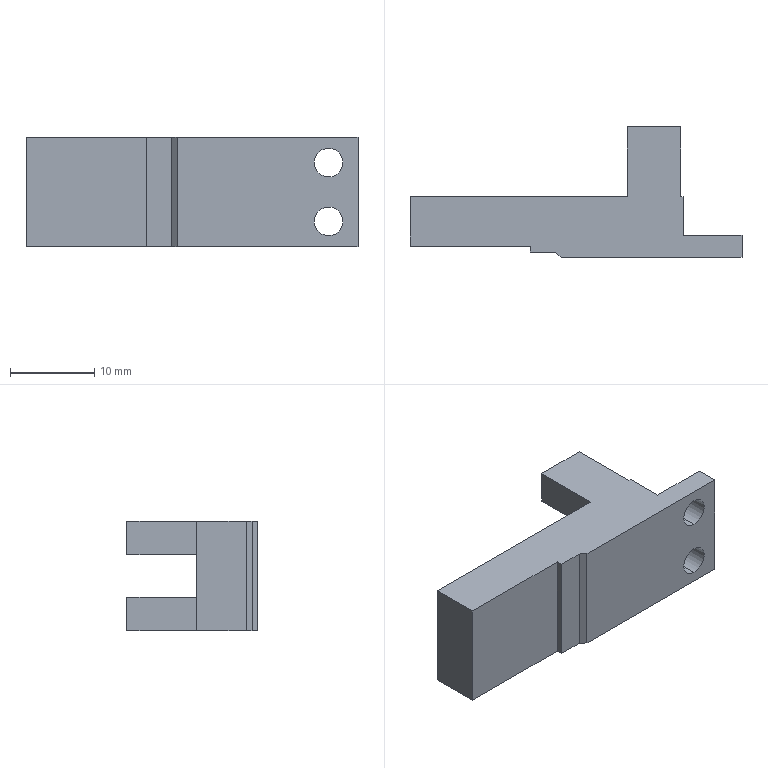Part | SolidWorks | features BaseBody 1 | 1 solid | 24 faces | box 39.5 x 15.5 x 13 mm | volume 3385 mm3 | plane 20 | cylinder 4 | commonest cylinder face diameters 3.4 x4
STEP:
#1=CARTESIAN_POINT('',(93.5,24.1,-79.8));
#2=VERTEX_POINT('',#1);
#3=CARTESIAN_POINT('',(93.5,24.1,-83.2));
#4=VERTEX_POINT('',#3);
#5=CARTESIAN_POINT('',(93.5,24.1,-81.5));
#6=DIRECTION('',(0.,-1.,0.));
#7=DIRECTION('',(0.,0.,-1.));
#8=AXIS2_PLACEMENT_3D('',#5,#6,#7);
#9=CIRCLE('',#8,1.7);
#10=EDGE_CURVE('',#2,#4,#9,.T.);
#11=ORIENTED_EDGE('',*,*,#10,.F.);
#12=CARTESIAN_POINT('',(93.5,21.5,-79.8));
#13=VERTEX_POINT('',#12);
#14=CARTESIAN_POINT('',(93.5,14.1,-79.8));
#15=DIRECTION('',(0.,-1.,0.));
#16=VECTOR('',#15,1000.);
#17=LINE('',#14,#16);
#18=EDGE_CURVE('',#2,#13,#17,.T.);
#19=ORIENTED_EDGE('',*,*,#18,.T.);
#20=CARTESIAN_POINT('',(93.5,21.5,-83.2));
#21=VERTEX_POINT('',#20);
#22=CARTESIAN_POINT('',(93.5,21.5,-81.5));
#23=DIRECTION('',(0.,1.,0.));
#24=DIRECTION('',(0.,0.,-1.));
#25=AXIS2_PLACEMENT_3D('',#22,#23,#24);
#26=CIRCLE('',#25,1.7);
#27=EDGE_CURVE('',#21,#13,#26,.T.);
#28=ORIENTED_EDGE('',*,*,#27,.F.);
#29=CARTESIAN_POINT('',(93.5,14.1,-83.2));
#30=DIRECTION('',(0.,-1.,0.));
#31=VECTOR('',#30,1000.);
#32=LINE('',#29,#31);
#33=EDGE_CURVE('',#4,#21,#32,.T.);
#34=ORIENTED_EDGE('',*,*,#33,.F.);
#35=EDGE_LOOP('',(#11,#19,#28,#34));
#36=FACE_OUTER_BOUND('',#35,.T.);
#37=CARTESIAN_POINT('',(93.5,14.1,-81.5));
#38=DIRECTION('',(0.,-1.,0.));
#39=DIRECTION('',(0.,0.,-1.));
#40=AXIS2_PLACEMENT_3D('',#37,#38,#39);
#41=CYLINDRICAL_SURFACE('',#40,1.7);
#42=ADVANCED_FACE('',(#36),#41,.F.);
#43=CARTESIAN_POINT('',(93.5,24.1,-72.8));
#44=VERTEX_POINT('',#43);
#45=CARTESIAN_POINT('',(93.5,24.1,-76.2));
#46=VERTEX_POINT('',#45);
#47=CARTESIAN_POINT('',(93.5,24.1,-74.5));
#48=DIRECTION('',(0.,-1.,0.));
#49=DIRECTION('',(0.,0.,-1.));
#50=AXIS2_PLACEMENT_3D('',#47,#48,#49);
#51=CIRCLE('',#50,1.7);
#52=EDGE_CURVE('',#44,#46,#51,.T.);
#53=ORIENTED_EDGE('',*,*,#52,.F.);
#54=CARTESIAN_POINT('',(93.5,21.5,-72.8));
#55=VERTEX_POINT('',#54);
#56=CARTESIAN_POINT('',(93.5,14.1,-72.8));
#57=DIRECTION('',(0.,-1.,0.));
#58=VECTOR('',#57,1000.);
#59=LINE('',#56,#58);
#60=EDGE_CURVE('',#44,#55,#59,.T.);
#61=ORIENTED_EDGE('',*,*,#60,.T.);
#62=CARTESIAN_POINT('',(93.5,21.5,-76.2));
#63=VERTEX_POINT('',#62);
#64=CARTESIAN_POINT('',(93.5,21.5,-74.5));
#65=DIRECTION('',(0.,1.,0.));
#66=DIRECTION('',(0.,0.,-1.));
#67=AXIS2_PLACEMENT_3D('',#64,#65,#66);
#68=CIRCLE('',#67,1.7);
#69=EDGE_CURVE('',#63,#55,#68,.T.);
#70=ORIENTED_EDGE('',*,*,#69,.F.);
#71=CARTESIAN_POINT('',(93.5,14.1,-76.2));
#72=DIRECTION('',(0.,-1.,0.));
#73=VECTOR('',#72,1000.);
#74=LINE('',#71,#73);
#75=EDGE_CURVE('',#46,#63,#74,.T.);
#76=ORIENTED_EDGE('',*,*,#75,.F.);
#77=EDGE_LOOP('',(#53,#61,#70,#76));
#78=FACE_OUTER_BOUND('',#77,.T.);
#79=CARTESIAN_POINT('',(93.5,14.1,-74.5));
#80=DIRECTION('',(0.,-1.,0.));
#81=DIRECTION('',(0.,0.,-1.));
#82=AXIS2_PLACEMENT_3D('',#79,#80,#81);
#83=CYLINDRICAL_SURFACE('',#82,1.7);
#84=ADVANCED_FACE('',(#78),#83,.F.);
#85=CARTESIAN_POINT('',(57.5,28.7,-84.5));
#86=VERTEX_POINT('',#85);
#87=CARTESIAN_POINT('',(57.5,28.7,-71.5));
#88=VERTEX_POINT('',#87);
#89=CARTESIAN_POINT('',(57.5,28.7,-84.5));
#90=DIRECTION('',(0.,0.,1.));
#91=VECTOR('',#90,1000.);
#92=LINE('',#89,#91);
#93=EDGE_CURVE('',#86,#88,#92,.T.);
#94=ORIENTED_EDGE('',*,*,#93,.T.);
#95=CARTESIAN_POINT('',(83.35,28.7,-71.5));
#96=VERTEX_POINT('',#95);
#97=CARTESIAN_POINT('',(83.35,28.7,-71.5));
#98=DIRECTION('',(1.,0.,0.));
#99=VECTOR('',#98,1000.);
#100=LINE('',#97,#99);
#101=EDGE_CURVE('',#88,#96,#100,.T.);
#102=ORIENTED_EDGE('',*,*,#101,.T.);
#103=CARTESIAN_POINT('',(83.35,28.7,-75.5));
#104=VERTEX_POINT('',#103);
#105=CARTESIAN_POINT('',(83.35,28.7,-84.5));
#106=DIRECTION('',(0.,0.,-1.));
#107=VECTOR('',#106,1000.);
#108=LINE('',#105,#107);
#109=EDGE_CURVE('',#96,#104,#108,.T.);
#110=ORIENTED_EDGE('',*,*,#109,.T.);
#111=CARTESIAN_POINT('',(89.7,28.7,-75.5));
#112=VERTEX_POINT('',#111);
#113=CARTESIAN_POINT('',(83.35,28.7,-75.5));
#114=DIRECTION('',(1.,0.,0.));
#115=VECTOR('',#114,1000.);
#116=LINE('',#113,#115);
#117=EDGE_CURVE('',#104,#112,#116,.T.);
#118=ORIENTED_EDGE('',*,*,#117,.T.);
#119=CARTESIAN_POINT('',(89.7,28.7,-71.5));
#120=VERTEX_POINT('',#119);
#121=CARTESIAN_POINT('',(89.7,28.7,-84.5));
#122=DIRECTION('',(0.,0.,1.));
#123=VECTOR('',#122,1000.);
#124=LINE('',#121,#123);
#125=EDGE_CURVE('',#112,#120,#124,.T.);
#126=ORIENTED_EDGE('',*,*,#125,.T.);
#127=CARTESIAN_POINT('',(90.,28.7,-71.5));
#128=VERTEX_POINT('',#127);
#129=CARTESIAN_POINT('',(83.35,28.7,-71.5));
#130=DIRECTION('',(1.,0.,0.));
#131=VECTOR('',#130,1000.);
#132=LINE('',#129,#131);
#133=EDGE_CURVE('',#120,#128,#132,.T.);
#134=ORIENTED_EDGE('',*,*,#133,.T.);
#135=CARTESIAN_POINT('',(90.,28.7,-84.5));
#136=VERTEX_POINT('',#135);
#137=CARTESIAN_POINT('',(90.,28.7,-84.5));
#138=DIRECTION('',(0.,0.,-1.));
#139=VECTOR('',#138,1000.);
#140=LINE('',#137,#139);
#141=EDGE_CURVE('',#128,#136,#140,.T.);
#142=ORIENTED_EDGE('',*,*,#141,.T.);
#143=CARTESIAN_POINT('',(89.7,28.7,-84.5));
#144=VERTEX_POINT('',#143);
#145=CARTESIAN_POINT('',(83.35,28.7,-84.5));
#146=DIRECTION('',(-1.,0.,0.));
#147=VECTOR('',#146,1000.);
#148=LINE('',#145,#147);
#149=EDGE_CURVE('',#136,#144,#148,.T.);
#150=ORIENTED_EDGE('',*,*,#149,.T.);
#151=CARTESIAN_POINT('',(89.7,28.7,-80.5));
#152=VERTEX_POINT('',#151);
#153=CARTESIAN_POINT('',(89.7,28.7,-84.5));
#154=DIRECTION('',(0.,0.,1.));
#155=VECTOR('',#154,1000.);
#156=LINE('',#153,#155);
#157=EDGE_CURVE('',#144,#152,#156,.T.);
#158=ORIENTED_EDGE('',*,*,#157,.T.);
#159=CARTESIAN_POINT('',(83.35,28.7,-80.5));
#160=VERTEX_POINT('',#159);
#161=CARTESIAN_POINT('',(83.35,28.7,-80.5));
#162=DIRECTION('',(-1.,0.,0.));
#163=VECTOR('',#162,1000.);
#164=LINE('',#161,#163);
#165=EDGE_CURVE('',#152,#160,#164,.T.);
#166=ORIENTED_EDGE('',*,*,#165,.T.);
#167=CARTESIAN_POINT('',(83.35,28.7,-84.5));
#168=VERTEX_POINT('',#167);
#169=CARTESIAN_POINT('',(83.35,28.7,-84.5));
#170=DIRECTION('',(0.,0.,-1.));
#171=VECTOR('',#170,1000.);
#172=LINE('',#169,#171);
#173=EDGE_CURVE('',#160,#168,#172,.T.);
#174=ORIENTED_EDGE('',*,*,#173,.T.);
#175=CARTESIAN_POINT('',(83.35,28.7,-84.5));
#176=DIRECTION('',(-1.,0.,0.));
#177=VECTOR('',#176,1000.);
#178=LINE('',#175,#177);
#179=EDGE_CURVE('',#168,#86,#178,.T.);
#180=ORIENTED_EDGE('',*,*,#179,.T.);
#181=EDGE_LOOP('',(#94,#102,#110,#118,#126,#134,#142,#150,#158,#166,#174,#180));
#182=FACE_OUTER_BOUND('',#181,.T.);
#183=CARTESIAN_POINT('',(83.35,28.7,-84.5));
#184=DIRECTION('',(0.,1.,0.));
#185=DIRECTION('',(0.,0.,1.));
#186=AXIS2_PLACEMENT_3D('',#183,#184,#185);
#187=PLANE('',#186);
#188=ADVANCED_FACE('',(#182),#187,.T.);
#189=CARTESIAN_POINT('',(83.35,37.,-71.5));
#190=VERTEX_POINT('',#189);
#191=CARTESIAN_POINT('',(83.35,0.,-71.5));
#192=DIRECTION('',(0.,-1.,0.));
#193=VECTOR('',#192,1000.);
#194=LINE('',#191,#193);
#195=EDGE_CURVE('',#190,#96,#194,.T.);
#196=ORIENTED_EDGE('',*,*,#195,.T.);
#197=ORIENTED_EDGE('',*,*,#101,.F.);
#198=CARTESIAN_POINT('',(57.5,22.8,-71.5));
#199=VERTEX_POINT('',#198);
#200=CARTESIAN_POINT('',(57.5,0.,-71.5));
#201=DIRECTION('',(0.,-1.,0.));
#202=VECTOR('',#201,1000.);
#203=LINE('',#200,#202);
#204=EDGE_CURVE('',#88,#199,#203,.T.);
#205=ORIENTED_EDGE('',*,*,#204,.T.);
#206=CARTESIAN_POINT('',(71.8,22.8,-71.5));
#207=VERTEX_POINT('',#206);
#208=CARTESIAN_POINT('',(0.,22.8,-71.5));
#209=DIRECTION('',(1.,0.,0.));
#210=VECTOR('',#209,1000.);
#211=LINE('',#208,#210);
#212=EDGE_CURVE('',#199,#207,#211,.T.);
#213=ORIENTED_EDGE('',*,*,#212,.T.);
#214=CARTESIAN_POINT('',(71.8,22.1,-71.5));
#215=VERTEX_POINT('',#214);
#216=CARTESIAN_POINT('',(71.8,22.8,-71.5));
#217=DIRECTION('',(0.,1.,0.));
#218=VECTOR('',#217,1000.);
#219=LINE('',#216,#218);
#220=EDGE_CURVE('',#215,#207,#219,.T.);
#221=ORIENTED_EDGE('',*,*,#220,.F.);
#222=CARTESIAN_POINT('',(74.8,22.1,-71.5));
#223=VERTEX_POINT('',#222);
#224=CARTESIAN_POINT('',(0.,22.1,-71.5));
#225=DIRECTION('',(1.,0.,0.));
#226=VECTOR('',#225,1000.);
#227=LINE('',#224,#226);
#228=EDGE_CURVE('',#215,#223,#227,.T.);
#229=ORIENTED_EDGE('',*,*,#228,.T.);
#230=CARTESIAN_POINT('',(75.5,21.5,-71.5));
#231=VERTEX_POINT('',#230);
#232=CARTESIAN_POINT('',(74.8,22.1,-71.5));
#233=DIRECTION('',(-0.7593,0.6508,0.));
#234=VECTOR('',#233,1000.);
#235=LINE('',#232,#234);
#236=EDGE_CURVE('',#231,#223,#235,.T.);
#237=ORIENTED_EDGE('',*,*,#236,.F.);
#238=CARTESIAN_POINT('',(97.,21.5,-71.5));
#239=VERTEX_POINT('',#238);
#240=CARTESIAN_POINT('',(0.,21.5,-71.5));
#241=DIRECTION('',(1.,0.,0.));
#242=VECTOR('',#241,1000.);
#243=LINE('',#240,#242);
#244=EDGE_CURVE('',#231,#239,#243,.T.);
#245=ORIENTED_EDGE('',*,*,#244,.T.);
#246=CARTESIAN_POINT('',(97.,24.1,-71.5));
#247=VERTEX_POINT('',#246);
#248=CARTESIAN_POINT('',(97.,0.,-71.5));
#249=DIRECTION('',(0.,1.,0.));
#250=VECTOR('',#249,1000.);
#251=LINE('',#248,#250);
#252=EDGE_CURVE('',#239,#247,#251,.T.);
#253=ORIENTED_EDGE('',*,*,#252,.T.);
#254=CARTESIAN_POINT('',(90.,24.1,-71.5));
#255=VERTEX_POINT('',#254);
#256=CARTESIAN_POINT('',(0.,24.1,-71.5));
#257=DIRECTION('',(-1.,0.,0.));
#258=VECTOR('',#257,1000.);
#259=LINE('',#256,#258);
#260=EDGE_CURVE('',#247,#255,#259,.T.);
#261=ORIENTED_EDGE('',*,*,#260,.T.);
#262=CARTESIAN_POINT('',(90.,0.,-71.5));
#263=DIRECTION('',(0.,1.,0.));
#264=VECTOR('',#263,1000.);
#265=LINE('',#262,#264);
#266=EDGE_CURVE('',#255,#128,#265,.T.);
#267=ORIENTED_EDGE('',*,*,#266,.T.);
#268=ORIENTED_EDGE('',*,*,#133,.F.);
#269=CARTESIAN_POINT('',(89.7,37.,-71.5));
#270=VERTEX_POINT('',#269);
#271=CARTESIAN_POINT('',(89.7,0.,-71.5));
#272=DIRECTION('',(0.,1.,0.));
#273=VECTOR('',#272,1000.);
#274=LINE('',#271,#273);
#275=EDGE_CURVE('',#120,#270,#274,.T.);
#276=ORIENTED_EDGE('',*,*,#275,.T.);
#277=CARTESIAN_POINT('',(0.,37.,-71.5));
#278=DIRECTION('',(-1.,0.,0.));
#279=VECTOR('',#278,1000.);
#280=LINE('',#277,#279);
#281=EDGE_CURVE('',#270,#190,#280,.T.);
#282=ORIENTED_EDGE('',*,*,#281,.T.);
#283=EDGE_LOOP('',(#196,#197,#205,#213,#221,#229,#237,#245,#253,#261,#267,#268,#276,#282));
#284=FACE_OUTER_BOUND('',#283,.T.);
#285=CARTESIAN_POINT('',(0.,0.,-71.5));
#286=DIRECTION('',(0.,0.,1.));
#287=DIRECTION('',(1.,0.,0.));
#288=AXIS2_PLACEMENT_3D('',#285,#286,#287);
#289=PLANE('',#288);
#290=ADVANCED_FACE('',(#284),#289,.T.);
#291=CARTESIAN_POINT('',(57.5,22.8,-84.5));
#292=VERTEX_POINT('',#291);
#293=CARTESIAN_POINT('',(57.5,28.7,-84.5));
#294=DIRECTION('',(0.,-1.,0.));
#295=VECTOR('',#294,1000.);
#296=LINE('',#293,#295);
#297=EDGE_CURVE('',#86,#292,#296,.T.);
#298=ORIENTED_EDGE('',*,*,#297,.T.);
#299=CARTESIAN_POINT('',(57.5,22.8,-84.5));
#300=DIRECTION('',(0.,0.,1.));
#301=VECTOR('',#300,1000.);
#302=LINE('',#299,#301);
#303=EDGE_CURVE('',#292,#199,#302,.T.);
#304=ORIENTED_EDGE('',*,*,#303,.T.);
#305=ORIENTED_EDGE('',*,*,#204,.F.);
#306=ORIENTED_EDGE('',*,*,#93,.F.);
#307=EDGE_LOOP('',(#298,#304,#305,#306));
#308=FACE_OUTER_BOUND('',#307,.T.);
#309=CARTESIAN_POINT('',(57.5,28.7,-84.5));
#310=DIRECTION('',(-1.,0.,0.));
#311=DIRECTION('',(0.,0.,1.));
#312=AXIS2_PLACEMENT_3D('',#309,#310,#311);
#313=PLANE('',#312);
#314=ADVANCED_FACE('',(#308),#313,.T.);
#315=ORIENTED_EDGE('',*,*,#179,.F.);
#316=CARTESIAN_POINT('',(83.35,37.,-84.5));
#317=VERTEX_POINT('',#316);
#318=CARTESIAN_POINT('',(83.35,0.,-84.5));
#319=DIRECTION('',(0.,-1.,0.));
#320=VECTOR('',#319,1000.);
#321=LINE('',#318,#320);
#322=EDGE_CURVE('',#317,#168,#321,.T.);
#323=ORIENTED_EDGE('',*,*,#322,.F.);
#324=CARTESIAN_POINT('',(89.7,37.,-84.5));
#325=VERTEX_POINT('',#324);
#326=CARTESIAN_POINT('',(0.,37.,-84.5));
#327=DIRECTION('',(-1.,0.,0.));
#328=VECTOR('',#327,1000.);
#329=LINE('',#326,#328);
#330=EDGE_CURVE('',#325,#317,#329,.T.);
#331=ORIENTED_EDGE('',*,*,#330,.F.);
#332=CARTESIAN_POINT('',(89.7,0.,-84.5));
#333=DIRECTION('',(0.,1.,0.));
#334=VECTOR('',#333,1000.);
#335=LINE('',#332,#334);
#336=EDGE_CURVE('',#144,#325,#335,.T.);
#337=ORIENTED_EDGE('',*,*,#336,.F.);
#338=ORIENTED_EDGE('',*,*,#149,.F.);
#339=CARTESIAN_POINT('',(90.,24.1,-84.5));
#340=VERTEX_POINT('',#339);
#341=CARTESIAN_POINT('',(90.,0.,-84.5));
#342=DIRECTION('',(0.,1.,0.));
#343=VECTOR('',#342,1000.);
#344=LINE('',#341,#343);
#345=EDGE_CURVE('',#340,#136,#344,.T.);
#346=ORIENTED_EDGE('',*,*,#345,.F.);
#347=CARTESIAN_POINT('',(97.,24.1,-84.5));
#348=VERTEX_POINT('',#347);
#349=CARTESIAN_POINT('',(0.,24.1,-84.5));
#350=DIRECTION('',(-1.,0.,0.));
#351=VECTOR('',#350,1000.);
#352=LINE('',#349,#351);
#353=EDGE_CURVE('',#348,#340,#352,.T.);
#354=ORIENTED_EDGE('',*,*,#353,.F.);
#355=CARTESIAN_POINT('',(97.,21.5,-84.5));
#356=VERTEX_POINT('',#355);
#357=CARTESIAN_POINT('',(97.,0.,-84.5));
#358=DIRECTION('',(0.,1.,0.));
#359=VECTOR('',#358,1000.);
#360=LINE('',#357,#359);
#361=EDGE_CURVE('',#356,#348,#360,.T.);
#362=ORIENTED_EDGE('',*,*,#361,.F.);
#363=CARTESIAN_POINT('',(75.5,21.5,-84.5));
#364=VERTEX_POINT('',#363);
#365=CARTESIAN_POINT('',(0.,21.5,-84.5));
#366=DIRECTION('',(1.,0.,0.));
#367=VECTOR('',#366,1000.);
#368=LINE('',#365,#367);
#369=EDGE_CURVE('',#364,#356,#368,.T.);
#370=ORIENTED_EDGE('',*,*,#369,.F.);
#371=CARTESIAN_POINT('',(74.8,22.1,-84.5));
#372=VERTEX_POINT('',#371);
#373=CARTESIAN_POINT('',(74.8,22.1,-84.5));
#374=DIRECTION('',(0.7593,-0.6508,0.));
#375=VECTOR('',#374,1000.);
#376=LINE('',#373,#375);
#377=EDGE_CURVE('',#372,#364,#376,.T.);
#378=ORIENTED_EDGE('',*,*,#377,.F.);
#379=CARTESIAN_POINT('',(71.8,22.1,-84.5));
#380=VERTEX_POINT('',#379);
#381=CARTESIAN_POINT('',(0.,22.1,-84.5));
#382=DIRECTION('',(1.,0.,0.));
#383=VECTOR('',#382,1000.);
#384=LINE('',#381,#383);
#385=EDGE_CURVE('',#380,#372,#384,.T.);
#386=ORIENTED_EDGE('',*,*,#385,.F.);
#387=CARTESIAN_POINT('',(71.8,22.8,-84.5));
#388=VERTEX_POINT('',#387);
#389=CARTESIAN_POINT('',(71.8,22.8,-84.5));
#390=DIRECTION('',(0.,-1.,0.));
#391=VECTOR('',#390,1000.);
#392=LINE('',#389,#391);
#393=EDGE_CURVE('',#388,#380,#392,.T.);
#394=ORIENTED_EDGE('',*,*,#393,.F.);
#395=CARTESIAN_POINT('',(0.,22.8,-84.5));
#396=DIRECTION('',(1.,0.,0.));
#397=VECTOR('',#396,1000.);
#398=LINE('',#395,#397);
#399=EDGE_CURVE('',#292,#388,#398,.T.);
#400=ORIENTED_EDGE('',*,*,#399,.F.);
#401=ORIENTED_EDGE('',*,*,#297,.F.);
#402=EDGE_LOOP('',(#315,#323,#331,#337,#338,#346,#354,#362,#370,#378,#386,#394,#400,#401));
#403=FACE_OUTER_BOUND('',#402,.T.);
#404=CARTESIAN_POINT('',(0.,0.,-84.5));
#405=DIRECTION('',(0.,0.,1.));
#406=DIRECTION('',(1.,0.,0.));
#407=AXIS2_PLACEMENT_3D('',#404,#405,#406);
#408=PLANE('',#407);
#409=ADVANCED_FACE('',(#403),#408,.F.);
#410=ORIENTED_EDGE('',*,*,#322,.T.);
#411=ORIENTED_EDGE('',*,*,#173,.F.);
#412=CARTESIAN_POINT('',(83.35,37.,-80.5));
#413=VERTEX_POINT('',#412);
#414=CARTESIAN_POINT('',(83.35,37.,-80.5));
#415=DIRECTION('',(0.,1.,0.));
#416=VECTOR('',#415,1000.);
#417=LINE('',#414,#416);
#418=EDGE_CURVE('',#160,#413,#417,.T.);
#419=ORIENTED_EDGE('',*,*,#418,.T.);
#420=CARTESIAN_POINT('',(83.35,37.,-84.5));
#421=DIRECTION('',(0.,0.,-1.));
#422=VECTOR('',#421,1000.);
#423=LINE('',#420,#422);
#424=EDGE_CURVE('',#413,#317,#423,.T.);
#425=ORIENTED_EDGE('',*,*,#424,.T.);
#426=EDGE_LOOP('',(#410,#411,#419,#425));
#427=FACE_OUTER_BOUND('',#426,.T.);
#428=CARTESIAN_POINT('',(83.35,37.,-84.5));
#429=DIRECTION('',(-1.,0.,0.));
#430=DIRECTION('',(0.,0.,1.));
#431=AXIS2_PLACEMENT_3D('',#428,#429,#430);
#432=PLANE('',#431);
#433=ADVANCED_FACE('',(#427),#432,.T.);
#434=ORIENTED_EDGE('',*,*,#165,.F.);
#435=CARTESIAN_POINT('',(89.7,37.,-80.5));
#436=VERTEX_POINT('',#435);
#437=CARTESIAN_POINT('',(89.7,28.7,-80.5));
#438=DIRECTION('',(0.,-1.,0.));
#439=VECTOR('',#438,1000.);
#440=LINE('',#437,#439);
#441=EDGE_CURVE('',#436,#152,#440,.T.);
#442=ORIENTED_EDGE('',*,*,#441,.F.);
#443=CARTESIAN_POINT('',(76.7,37.,-80.5));
#444=DIRECTION('',(1.,0.,0.));
#445=VECTOR('',#444,1000.);
#446=LINE('',#443,#445);
#447=EDGE_CURVE('',#413,#436,#446,.T.);
#448=ORIENTED_EDGE('',*,*,#447,.F.);
#449=ORIENTED_EDGE('',*,*,#418,.F.);
#450=EDGE_LOOP('',(#434,#442,#448,#449));
#451=FACE_OUTER_BOUND('',#450,.T.);
#452=CARTESIAN_POINT('',(76.7,28.7,-80.5));
#453=DIRECTION('',(0.,0.,-1.));
#454=DIRECTION('',(-1.,0.,0.));
#455=AXIS2_PLACEMENT_3D('',#452,#453,#454);
#456=PLANE('',#455);
#457=ADVANCED_FACE('',(#451),#456,.F.);
#458=ORIENTED_EDGE('',*,*,#336,.T.);
#459=CARTESIAN_POINT('',(89.7,37.,-84.5));
#460=DIRECTION('',(0.,0.,1.));
#461=VECTOR('',#460,1000.);
#462=LINE('',#459,#461);
#463=EDGE_CURVE('',#325,#436,#462,.T.);
#464=ORIENTED_EDGE('',*,*,#463,.T.);
#465=ORIENTED_EDGE('',*,*,#441,.T.);
#466=ORIENTED_EDGE('',*,*,#157,.F.);
#467=EDGE_LOOP('',(#458,#464,#465,#466));
#468=FACE_OUTER_BOUND('',#467,.T.);
#469=CARTESIAN_POINT('',(89.7,28.7,-84.5));
#470=DIRECTION('',(1.,0.,0.));
#471=DIRECTION('',(0.,0.,-1.));
#472=AXIS2_PLACEMENT_3D('',#469,#470,#471);
#473=PLANE('',#472);
#474=ADVANCED_FACE('',(#468),#473,.T.);
#475=ORIENTED_EDGE('',*,*,#345,.T.);
#476=ORIENTED_EDGE('',*,*,#141,.F.);
#477=ORIENTED_EDGE('',*,*,#266,.F.);
#478=CARTESIAN_POINT('',(90.,24.1,-84.5));
#479=DIRECTION('',(0.,0.,-1.));
#480=VECTOR('',#479,1000.);
#481=LINE('',#478,#480);
#482=EDGE_CURVE('',#255,#340,#481,.T.);
#483=ORIENTED_EDGE('',*,*,#482,.T.);
#484=EDGE_LOOP('',(#475,#476,#477,#483));
#485=FACE_OUTER_BOUND('',#484,.T.);
#486=CARTESIAN_POINT('',(90.,24.1,-84.5));
#487=DIRECTION('',(1.,0.,0.));
#488=DIRECTION('',(0.,0.,-1.));
#489=AXIS2_PLACEMENT_3D('',#486,#487,#488);
#490=PLANE('',#489);
#491=ADVANCED_FACE('',(#485),#490,.T.);
#492=ORIENTED_EDGE('',*,*,#275,.F.);
#493=ORIENTED_EDGE('',*,*,#125,.F.);
#494=CARTESIAN_POINT('',(89.7,37.,-75.5));
#495=VERTEX_POINT('',#494);
#496=CARTESIAN_POINT('',(89.7,28.7,-75.5));
#497=DIRECTION('',(0.,1.,0.));
#498=VECTOR('',#497,1000.);
#499=LINE('',#496,#498);
#500=EDGE_CURVE('',#112,#495,#499,.T.);
#501=ORIENTED_EDGE('',*,*,#500,.T.);
#502=CARTESIAN_POINT('',(89.7,37.,-84.5));
#503=DIRECTION('',(0.,0.,1.));
#504=VECTOR('',#503,1000.);
#505=LINE('',#502,#504);
#506=EDGE_CURVE('',#495,#270,#505,.T.);
#507=ORIENTED_EDGE('',*,*,#506,.T.);
#508=EDGE_LOOP('',(#492,#493,#501,#507));
#509=FACE_OUTER_BOUND('',#508,.T.);
#510=CARTESIAN_POINT('',(89.7,28.7,-84.5));
#511=DIRECTION('',(1.,0.,0.));
#512=DIRECTION('',(0.,0.,-1.));
#513=AXIS2_PLACEMENT_3D('',#510,#511,#512);
#514=PLANE('',#513);
#515=ADVANCED_FACE('',(#509),#514,.T.);
#516=CARTESIAN_POINT('',(83.35,37.,-75.5));
#517=VERTEX_POINT('',#516);
#518=CARTESIAN_POINT('',(76.7,37.,-75.5));
#519=DIRECTION('',(-1.,0.,0.));
#520=VECTOR('',#519,1000.);
#521=LINE('',#518,#520);
#522=EDGE_CURVE('',#495,#517,#521,.T.);
#523=ORIENTED_EDGE('',*,*,#522,.F.);
#524=ORIENTED_EDGE('',*,*,#500,.F.);
#525=ORIENTED_EDGE('',*,*,#117,.F.);
#526=CARTESIAN_POINT('',(83.35,37.,-75.5));
#527=DIRECTION('',(0.,-1.,0.));
#528=VECTOR('',#527,1000.);
#529=LINE('',#526,#528);
#530=EDGE_CURVE('',#517,#104,#529,.T.);
#531=ORIENTED_EDGE('',*,*,#530,.F.);
#532=EDGE_LOOP('',(#523,#524,#525,#531));
#533=FACE_OUTER_BOUND('',#532,.T.);
#534=CARTESIAN_POINT('',(76.7,37.,-75.5));
#535=DIRECTION('',(0.,0.,1.));
#536=DIRECTION('',(1.,0.,0.));
#537=AXIS2_PLACEMENT_3D('',#534,#535,#536);
#538=PLANE('',#537);
#539=ADVANCED_FACE('',(#533),#538,.F.);
#540=ORIENTED_EDGE('',*,*,#195,.F.);
#541=CARTESIAN_POINT('',(83.35,37.,-84.5));
#542=DIRECTION('',(0.,0.,-1.));
#543=VECTOR('',#542,1000.);
#544=LINE('',#541,#543);
#545=EDGE_CURVE('',#190,#517,#544,.T.);
#546=ORIENTED_EDGE('',*,*,#545,.T.);
#547=ORIENTED_EDGE('',*,*,#530,.T.);
#548=ORIENTED_EDGE('',*,*,#109,.F.);
#549=EDGE_LOOP('',(#540,#546,#547,#548));
#550=FACE_OUTER_BOUND('',#549,.T.);
#551=CARTESIAN_POINT('',(83.35,37.,-84.5));
#552=DIRECTION('',(-1.,0.,0.));
#553=DIRECTION('',(0.,0.,1.));
#554=AXIS2_PLACEMENT_3D('',#551,#552,#553);
#555=PLANE('',#554);
#556=ADVANCED_FACE('',(#550),#555,.T.);
#557=ORIENTED_EDGE('',*,*,#281,.F.);
#558=ORIENTED_EDGE('',*,*,#506,.F.);
#559=ORIENTED_EDGE('',*,*,#522,.T.);
#560=ORIENTED_EDGE('',*,*,#545,.F.);
#561=EDGE_LOOP('',(#557,#558,#559,#560));
#562=FACE_OUTER_BOUND('',#561,.T.);
#563=CARTESIAN_POINT('',(89.7,37.,-84.5));
#564=DIRECTION('',(0.,1.,0.));
#565=DIRECTION('',(0.,0.,1.));
#566=AXIS2_PLACEMENT_3D('',#563,#564,#565);
#567=PLANE('',#566);
#568=ADVANCED_FACE('',(#562),#567,.T.);
#569=ORIENTED_EDGE('',*,*,#353,.T.);
#570=ORIENTED_EDGE('',*,*,#482,.F.);
#571=ORIENTED_EDGE('',*,*,#260,.F.);
#572=CARTESIAN_POINT('',(97.,24.1,-84.5));
#573=DIRECTION('',(0.,0.,-1.));
#574=VECTOR('',#573,1000.);
#575=LINE('',#572,#574);
#576=EDGE_CURVE('',#247,#348,#575,.T.);
#577=ORIENTED_EDGE('',*,*,#576,.T.);
#578=EDGE_LOOP('',(#569,#570,#571,#577));
#579=FACE_OUTER_BOUND('',#578,.T.);
#580=CARTESIAN_POINT('',(93.5,24.1,-81.5));
#581=DIRECTION('',(0.,-1.,0.));
#582=DIRECTION('',(0.,0.,-1.));
#583=AXIS2_PLACEMENT_3D('',#580,#581,#582);
#584=CIRCLE('',#583,1.7);
#585=EDGE_CURVE('',#4,#2,#584,.T.);
#586=ORIENTED_EDGE('',*,*,#585,.T.);
#587=ORIENTED_EDGE('',*,*,#10,.T.);
#588=EDGE_LOOP('',(#586,#587));
#589=FACE_BOUND('',#588,.T.);
#590=CARTESIAN_POINT('',(93.5,24.1,-74.5));
#591=DIRECTION('',(0.,-1.,0.));
#592=DIRECTION('',(0.,0.,-1.));
#593=AXIS2_PLACEMENT_3D('',#590,#591,#592);
#594=CIRCLE('',#593,1.7);
#595=EDGE_CURVE('',#46,#44,#594,.T.);
#596=ORIENTED_EDGE('',*,*,#595,.T.);
#597=ORIENTED_EDGE('',*,*,#52,.T.);
#598=EDGE_LOOP('',(#596,#597));
#599=FACE_BOUND('',#598,.T.);
#600=CARTESIAN_POINT('',(97.,24.1,-84.5));
#601=DIRECTION('',(0.,1.,0.));
#602=DIRECTION('',(0.,0.,1.));
#603=AXIS2_PLACEMENT_3D('',#600,#601,#602);
#604=PLANE('',#603);
#605=ADVANCED_FACE('',(#579,#589,#599),#604,.T.);
#606=ORIENTED_EDGE('',*,*,#361,.T.);
#607=ORIENTED_EDGE('',*,*,#576,.F.);
#608=ORIENTED_EDGE('',*,*,#252,.F.);
#609=CARTESIAN_POINT('',(97.,21.5,-84.5));
#610=DIRECTION('',(0.,0.,-1.));
#611=VECTOR('',#610,1000.);
#612=LINE('',#609,#611);
#613=EDGE_CURVE('',#239,#356,#612,.T.);
#614=ORIENTED_EDGE('',*,*,#613,.T.);
#615=EDGE_LOOP('',(#606,#607,#608,#614));
#616=FACE_OUTER_BOUND('',#615,.T.);
#617=CARTESIAN_POINT('',(97.,21.5,-84.5));
#618=DIRECTION('',(1.,0.,0.));
#619=DIRECTION('',(0.,0.,-1.));
#620=AXIS2_PLACEMENT_3D('',#617,#618,#619);
#621=PLANE('',#620);
#622=ADVANCED_FACE('',(#616),#621,.T.);
#623=ORIENTED_EDGE('',*,*,#369,.T.);
#624=ORIENTED_EDGE('',*,*,#613,.F.);
#625=ORIENTED_EDGE('',*,*,#244,.F.);
#626=CARTESIAN_POINT('',(75.5,21.5,-84.5));
#627=DIRECTION('',(0.,0.,-1.));
#628=VECTOR('',#627,1000.);
#629=LINE('',#626,#628);
#630=EDGE_CURVE('',#231,#364,#629,.T.);
#631=ORIENTED_EDGE('',*,*,#630,.T.);
#632=EDGE_LOOP('',(#623,#624,#625,#631));
#633=FACE_OUTER_BOUND('',#632,.T.);
#634=ORIENTED_EDGE('',*,*,#27,.T.);
#635=CARTESIAN_POINT('',(93.5,21.5,-81.5));
#636=DIRECTION('',(0.,1.,0.));
#637=DIRECTION('',(0.,0.,-1.));
#638=AXIS2_PLACEMENT_3D('',#635,#636,#637);
#639=CIRCLE('',#638,1.7);
#640=EDGE_CURVE('',#13,#21,#639,.T.);
#641=ORIENTED_EDGE('',*,*,#640,.T.);
#642=EDGE_LOOP('',(#634,#641));
#643=FACE_BOUND('',#642,.T.);
#644=ORIENTED_EDGE('',*,*,#69,.T.);
#645=CARTESIAN_POINT('',(93.5,21.5,-74.5));
#646=DIRECTION('',(0.,1.,0.));
#647=DIRECTION('',(0.,0.,-1.));
#648=AXIS2_PLACEMENT_3D('',#645,#646,#647);
#649=CIRCLE('',#648,1.7);
#650=EDGE_CURVE('',#55,#63,#649,.T.);
#651=ORIENTED_EDGE('',*,*,#650,.T.);
#652=EDGE_LOOP('',(#644,#651));
#653=FACE_BOUND('',#652,.T.);
#654=CARTESIAN_POINT('',(75.5,21.5,-84.5));
#655=DIRECTION('',(0.,-1.,0.));
#656=DIRECTION('',(0.,0.,-1.));
#657=AXIS2_PLACEMENT_3D('',#654,#655,#656);
#658=PLANE('',#657);
#659=ADVANCED_FACE('',(#633,#643,#653),#658,.T.);
#660=ORIENTED_EDGE('',*,*,#385,.T.);
#661=CARTESIAN_POINT('',(74.8,22.1,-84.5));
#662=DIRECTION('',(0.,0.,1.));
#663=VECTOR('',#662,1000.);
#664=LINE('',#661,#663);
#665=EDGE_CURVE('',#372,#223,#664,.T.);
#666=ORIENTED_EDGE('',*,*,#665,.T.);
#667=ORIENTED_EDGE('',*,*,#228,.F.);
#668=CARTESIAN_POINT('',(71.8,22.1,-84.5));
#669=DIRECTION('',(0.,0.,-1.));
#670=VECTOR('',#669,1000.);
#671=LINE('',#668,#670);
#672=EDGE_CURVE('',#215,#380,#671,.T.);
#673=ORIENTED_EDGE('',*,*,#672,.T.);
#674=EDGE_LOOP('',(#660,#666,#667,#673));
#675=FACE_OUTER_BOUND('',#674,.T.);
#676=CARTESIAN_POINT('',(71.8,22.1,-84.5));
#677=DIRECTION('',(0.,-1.,0.));
#678=DIRECTION('',(0.,0.,-1.));
#679=AXIS2_PLACEMENT_3D('',#676,#677,#678);
#680=PLANE('',#679);
#681=ADVANCED_FACE('',(#675),#680,.T.);
#682=ORIENTED_EDGE('',*,*,#399,.T.);
#683=CARTESIAN_POINT('',(71.8,22.8,-84.5));
#684=DIRECTION('',(0.,0.,1.));
#685=VECTOR('',#684,1000.);
#686=LINE('',#683,#685);
#687=EDGE_CURVE('',#388,#207,#686,.T.);
#688=ORIENTED_EDGE('',*,*,#687,.T.);
#689=ORIENTED_EDGE('',*,*,#212,.F.);
#690=ORIENTED_EDGE('',*,*,#303,.F.);
#691=EDGE_LOOP('',(#682,#688,#689,#690));
#692=FACE_OUTER_BOUND('',#691,.T.);
#693=CARTESIAN_POINT('',(57.5,22.8,-84.5));
#694=DIRECTION('',(0.,-1.,0.));
#695=DIRECTION('',(0.,0.,-1.));
#696=AXIS2_PLACEMENT_3D('',#693,#694,#695);
#697=PLANE('',#696);
#698=ADVANCED_FACE('',(#692),#697,.T.);
#699=ORIENTED_EDGE('',*,*,#330,.T.);
#700=ORIENTED_EDGE('',*,*,#424,.F.);
#701=ORIENTED_EDGE('',*,*,#447,.T.);
#702=ORIENTED_EDGE('',*,*,#463,.F.);
#703=EDGE_LOOP('',(#699,#700,#701,#702));
#704=FACE_OUTER_BOUND('',#703,.T.);
#705=CARTESIAN_POINT('',(89.7,37.,-84.5));
#706=DIRECTION('',(0.,1.,0.));
#707=DIRECTION('',(0.,0.,1.));
#708=AXIS2_PLACEMENT_3D('',#705,#706,#707);
#709=PLANE('',#708);
#710=ADVANCED_FACE('',(#704),#709,.T.);
#711=ORIENTED_EDGE('',*,*,#18,.F.);
#712=ORIENTED_EDGE('',*,*,#585,.F.);
#713=ORIENTED_EDGE('',*,*,#33,.T.);
#714=ORIENTED_EDGE('',*,*,#640,.F.);
#715=EDGE_LOOP('',(#711,#712,#713,#714));
#716=FACE_OUTER_BOUND('',#715,.T.);
#717=CARTESIAN_POINT('',(93.5,14.1,-81.5));
#718=DIRECTION('',(0.,-1.,0.));
#719=DIRECTION('',(0.,0.,-1.));
#720=AXIS2_PLACEMENT_3D('',#717,#718,#719);
#721=CYLINDRICAL_SURFACE('',#720,1.7);
#722=ADVANCED_FACE('',(#716),#721,.F.);
#723=ORIENTED_EDGE('',*,*,#60,.F.);
#724=ORIENTED_EDGE('',*,*,#595,.F.);
#725=ORIENTED_EDGE('',*,*,#75,.T.);
#726=ORIENTED_EDGE('',*,*,#650,.F.);
#727=EDGE_LOOP('',(#723,#724,#725,#726));
#728=FACE_OUTER_BOUND('',#727,.T.);
#729=CARTESIAN_POINT('',(93.5,14.1,-74.5));
#730=DIRECTION('',(0.,-1.,0.));
#731=DIRECTION('',(0.,0.,-1.));
#732=AXIS2_PLACEMENT_3D('',#729,#730,#731);
#733=CYLINDRICAL_SURFACE('',#732,1.7);
#734=ADVANCED_FACE('',(#728),#733,.F.);
#735=ORIENTED_EDGE('',*,*,#377,.T.);
#736=ORIENTED_EDGE('',*,*,#630,.F.);
#737=ORIENTED_EDGE('',*,*,#236,.T.);
#738=ORIENTED_EDGE('',*,*,#665,.F.);
#739=EDGE_LOOP('',(#735,#736,#737,#738));
#740=FACE_OUTER_BOUND('',#739,.T.);
#741=CARTESIAN_POINT('',(74.8,22.1,-84.5));
#742=DIRECTION('',(-0.6508,-0.7593,0.));
#743=DIRECTION('',(0.7593,-0.6508,0.));
#744=AXIS2_PLACEMENT_3D('',#741,#742,#743);
#745=PLANE('',#744);
#746=ADVANCED_FACE('',(#740),#745,.T.);
#747=ORIENTED_EDGE('',*,*,#393,.T.);
#748=ORIENTED_EDGE('',*,*,#672,.F.);
#749=ORIENTED_EDGE('',*,*,#220,.T.);
#750=ORIENTED_EDGE('',*,*,#687,.F.);
#751=EDGE_LOOP('',(#747,#748,#749,#750));
#752=FACE_OUTER_BOUND('',#751,.T.);
#753=CARTESIAN_POINT('',(71.8,22.8,-84.5));
#754=DIRECTION('',(-1.,0.,0.));
#755=DIRECTION('',(0.,0.,1.));
#756=AXIS2_PLACEMENT_3D('',#753,#754,#755);
#757=PLANE('',#756);
#758=ADVANCED_FACE('',(#752),#757,.T.);
#759=CLOSED_SHELL('',(#42,#84,#188,#290,#314,#409,#433,#457,#474,#491,#515,#539,#556,#568,#605,#622,#659,#681,#698,#710,#722,#734,#746,#758));
#760=MANIFOLD_SOLID_BREP('',#759);
#761=CARTESIAN_POINT('',(0.,0.,0.));
#762=DIRECTION('',(0.,0.,1.));
#763=DIRECTION('',(1.,0.,0.));
#764=AXIS2_PLACEMENT_3D('',#761,#762,#763);
#765=(LENGTH_UNIT()NAMED_UNIT(*)SI_UNIT(.MILLI.,.METRE.));
#766=UNCERTAINTY_MEASURE_WITH_UNIT(LENGTH_MEASURE(0.00001),#765,'','');
#767=(NAMED_UNIT(*)PLANE_ANGLE_UNIT()SI_UNIT($,.RADIAN.));
#768=(NAMED_UNIT(*)SI_UNIT($,.STERADIAN.)SOLID_ANGLE_UNIT());
#769=(GEOMETRIC_REPRESENTATION_CONTEXT(3)GLOBAL_UNCERTAINTY_ASSIGNED_CONTEXT((#766))GLOBAL_UNIT_ASSIGNED_CONTEXT((#765,#767,#768))REPRESENTATION_CONTEXT('',''));
#770=ADVANCED_BREP_SHAPE_REPRESENTATION('',(#760,#764),#769);